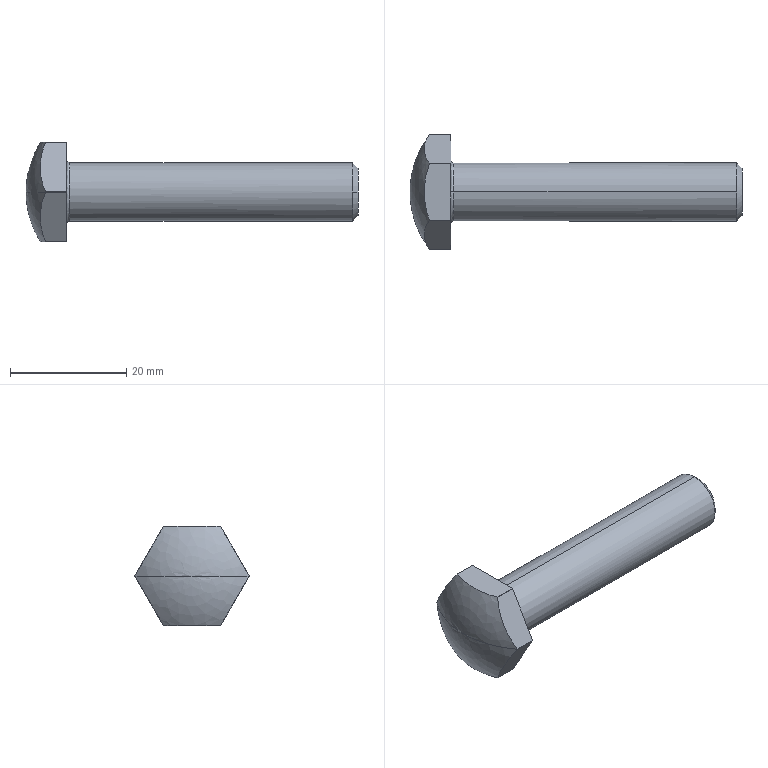Part | STEP file | 1_5 | 1 solid | 22 faces | volume 5335 mm3 | cylinder 8 | plane 8 | spline 4 | cone 2 | commonest cylinder face diameters 19.6 x6 10 x2